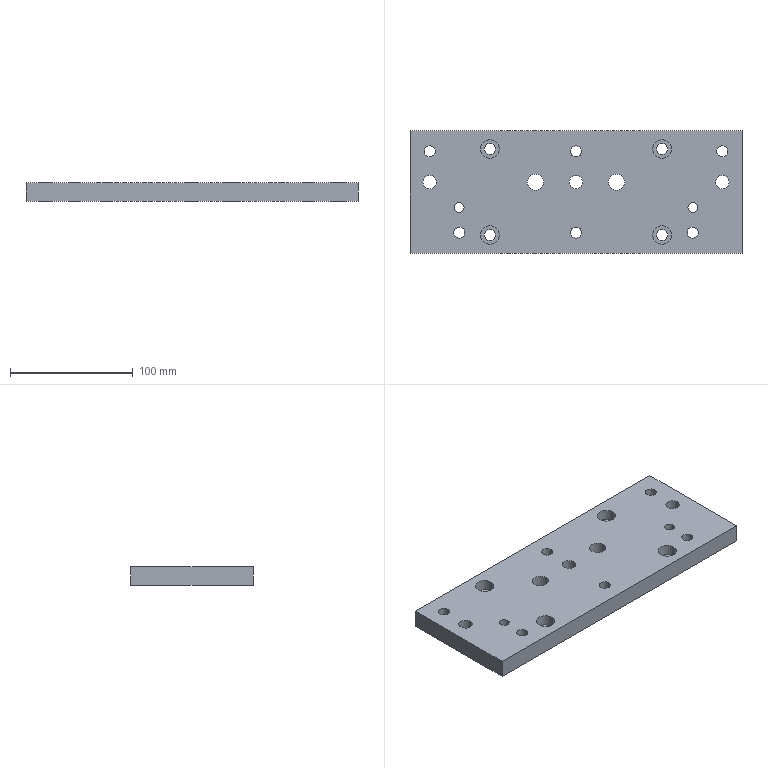Part | STEP file | TAM LOT CHAY | 1 solid | 52 faces | box 270 x 100 x 15 mm | volume 381434 mm3 | cylinder 42 | plane 10 | commonest cylinder face diameters 9 x20 15 x8 11 x6 8 x4 13.3 x4